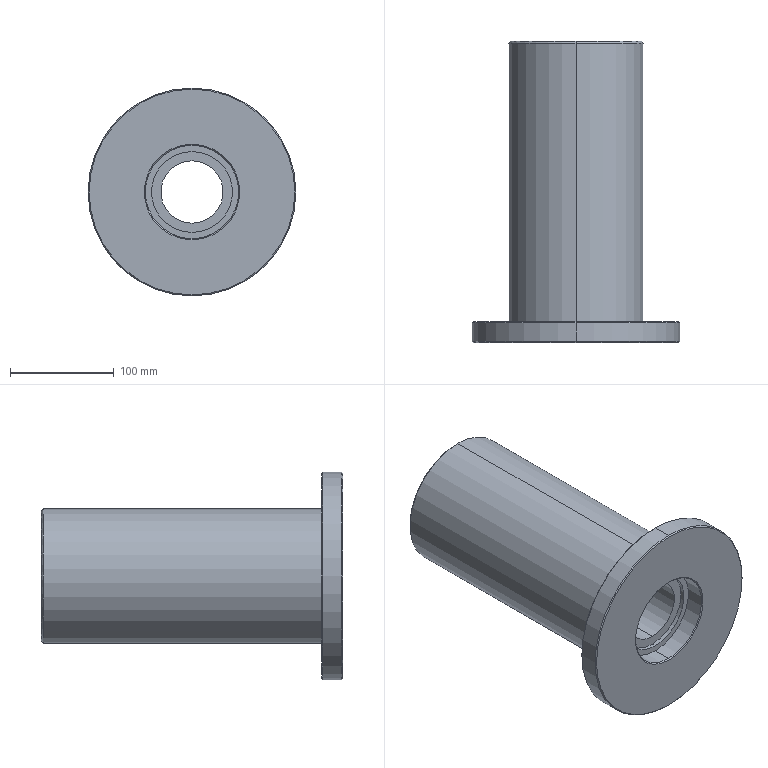Part | STEP file | Backup 2012-3-22-03 | 1 solid | 31 faces | box 200 x 290 x 200 mm | volume 3240505 mm3 | cylinder 14 | cone 10 | plane 7 | commonest cylinder face diameters 78 x4 90 x4 60 x2 130 x2 200 x2